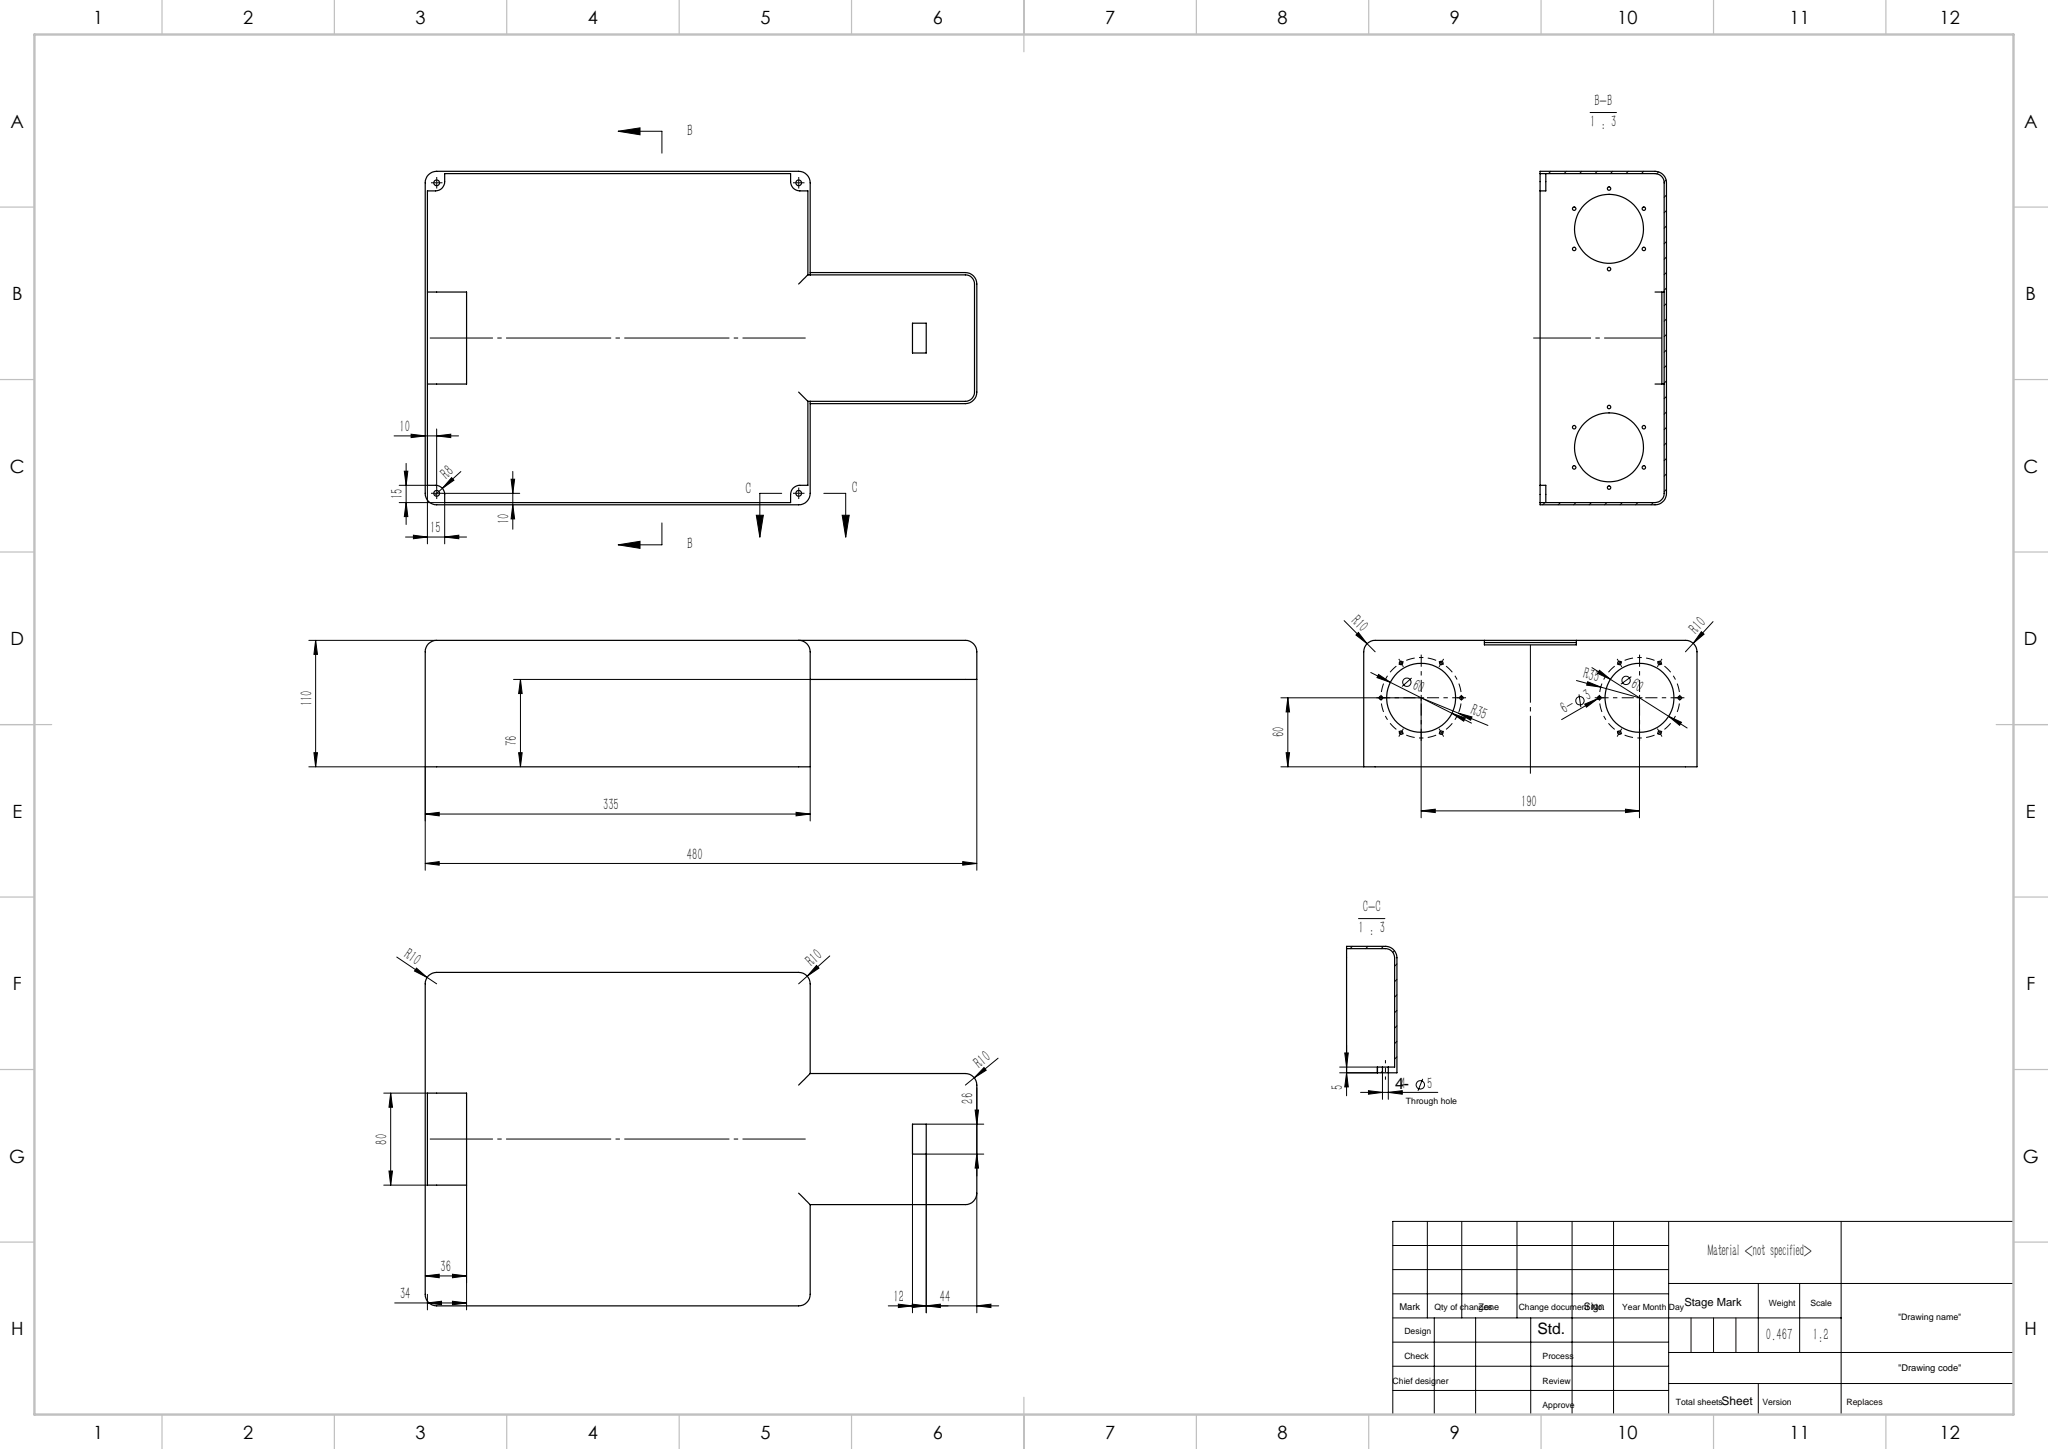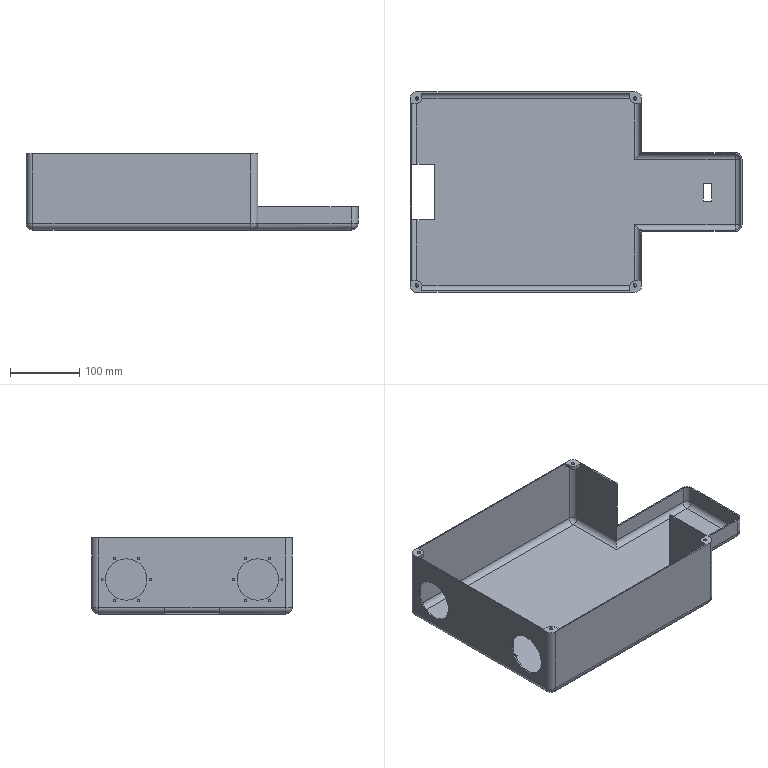Part | SolidWorks | features ICE 6, Fillet 3, CirPattern 2, Extrusion 1, Shell 1 | 1 solid | 120 faces | box 480 x 290 x 110 mm | volume 467348 mm3 | cylinder 69 | plane 39 | sphere 12 | commonest cylinder face diameters 3 x24 16 x19 20 x14 5 x8 60 x4